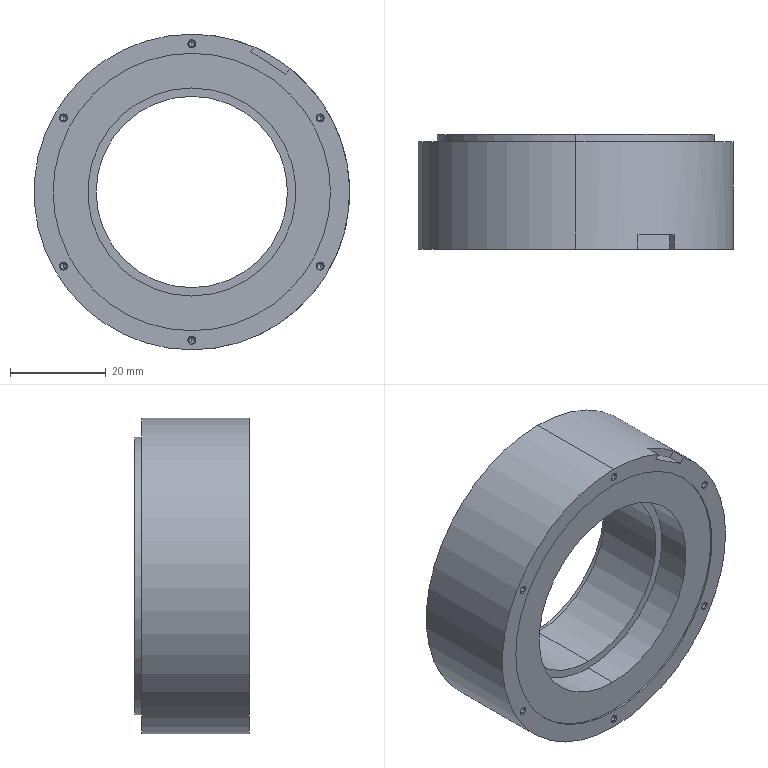Part | SolidWorks | features ICE 7, HoleWzd 2, Extrusion 1 | 1 solid | 88 faces | box 66 x 24 x 66 mm | volume 48084 mm3 | cone 40 | cylinder 36 | plane 12 | commonest cylinder face diameters 1.25 x12 2.5 x8 4 x4 58 x4 40 x2 42 x2